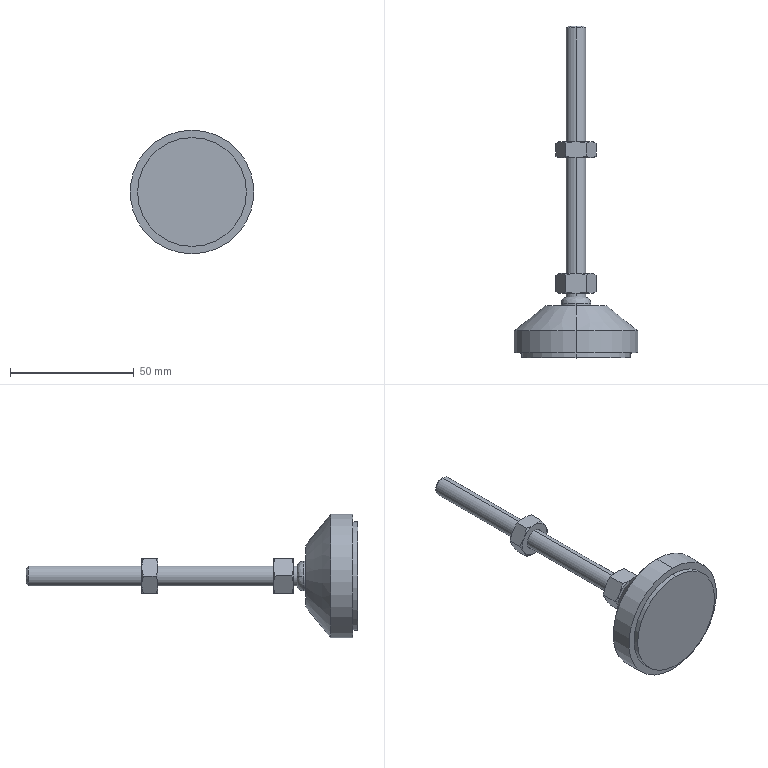Part | SolidWorks | features BaseBody 2 | 2 solids | 68 faces | box 50 x 134.1 x 50 mm | volume 39920 mm3 | cone 34 | plane 20 | cylinder 12 | spline 2 | commonest cylinder face diameters 8 x4 6.88 x2 12 x2 44 x2 50 x2